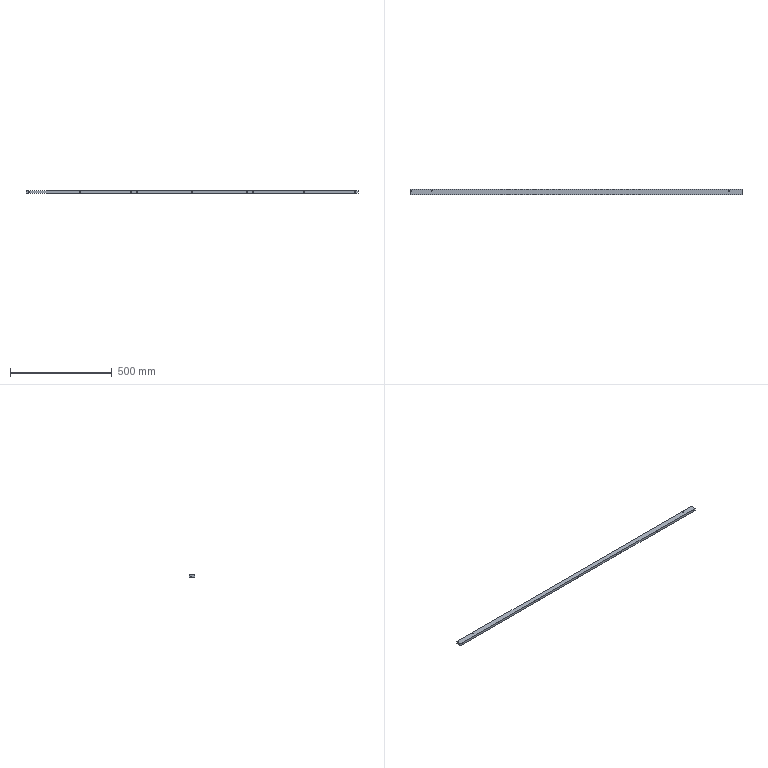Part | STEP file | J013-EBZ05-10-06 | 1 solid | 30 faces | box 1630 x 25 x 12 mm | volume 483875 mm3 | cylinder 24 | plane 6 | commonest cylinder face diameters 5 x24
STEP:
#1=CARTESIAN_POINT('',(1612.5,25.,6.));
#2=VERTEX_POINT('',#1);
#3=CARTESIAN_POINT('',(1617.5,25.,6.));
#4=VERTEX_POINT('',#3);
#5=CARTESIAN_POINT('',(1615.,25.,6.));
#6=DIRECTION('',(0.,-1.,0.));
#7=DIRECTION('',(1.,0.,0.));
#8=AXIS2_PLACEMENT_3D('',#5,#6,#7);
#9=CIRCLE('',#8,2.5);
#10=EDGE_CURVE('',#2,#4,#9,.T.);
#11=ORIENTED_EDGE('',*,*,#10,.F.);
#12=CARTESIAN_POINT('',(1612.5,0.,6.));
#13=VERTEX_POINT('',#12);
#14=CARTESIAN_POINT('',(1612.5,25.,6.));
#15=DIRECTION('',(0.,-1.,0.));
#16=VECTOR('',#15,1000.);
#17=LINE('',#14,#16);
#18=EDGE_CURVE('',#2,#13,#17,.T.);
#19=ORIENTED_EDGE('',*,*,#18,.T.);
#20=CARTESIAN_POINT('',(1617.5,0.,6.));
#21=VERTEX_POINT('',#20);
#22=CARTESIAN_POINT('',(1615.,0.,6.));
#23=DIRECTION('',(0.,1.,0.));
#24=DIRECTION('',(-1.,0.,0.));
#25=AXIS2_PLACEMENT_3D('',#22,#23,#24);
#26=CIRCLE('',#25,2.5);
#27=EDGE_CURVE('',#21,#13,#26,.T.);
#28=ORIENTED_EDGE('',*,*,#27,.F.);
#29=CARTESIAN_POINT('',(1617.5,25.,6.));
#30=DIRECTION('',(0.,-1.,0.));
#31=VECTOR('',#30,1000.);
#32=LINE('',#29,#31);
#33=EDGE_CURVE('',#4,#21,#32,.T.);
#34=ORIENTED_EDGE('',*,*,#33,.F.);
#35=EDGE_LOOP('',(#11,#19,#28,#34));
#36=FACE_OUTER_BOUND('',#35,.T.);
#37=CARTESIAN_POINT('',(1615.,25.,6.));
#38=DIRECTION('',(0.,-1.,0.));
#39=DIRECTION('',(1.,0.,0.));
#40=AXIS2_PLACEMENT_3D('',#37,#38,#39);
#41=CYLINDRICAL_SURFACE('',#40,2.5);
#42=ADVANCED_FACE('',(#36),#41,.F.);
#43=CARTESIAN_POINT('',(1362.5,25.,6.));
#44=VERTEX_POINT('',#43);
#45=CARTESIAN_POINT('',(1367.5,25.,6.));
#46=VERTEX_POINT('',#45);
#47=CARTESIAN_POINT('',(1365.,25.,6.));
#48=DIRECTION('',(0.,-1.,0.));
#49=DIRECTION('',(1.,0.,0.));
#50=AXIS2_PLACEMENT_3D('',#47,#48,#49);
#51=CIRCLE('',#50,2.5);
#52=EDGE_CURVE('',#44,#46,#51,.T.);
#53=ORIENTED_EDGE('',*,*,#52,.F.);
#54=CARTESIAN_POINT('',(1362.5,0.,6.));
#55=VERTEX_POINT('',#54);
#56=CARTESIAN_POINT('',(1362.5,25.,6.));
#57=DIRECTION('',(0.,-1.,0.));
#58=VECTOR('',#57,1000.);
#59=LINE('',#56,#58);
#60=EDGE_CURVE('',#44,#55,#59,.T.);
#61=ORIENTED_EDGE('',*,*,#60,.T.);
#62=CARTESIAN_POINT('',(1367.5,0.,6.));
#63=VERTEX_POINT('',#62);
#64=CARTESIAN_POINT('',(1365.,0.,6.));
#65=DIRECTION('',(0.,1.,0.));
#66=DIRECTION('',(-1.,0.,0.));
#67=AXIS2_PLACEMENT_3D('',#64,#65,#66);
#68=CIRCLE('',#67,2.5);
#69=EDGE_CURVE('',#63,#55,#68,.T.);
#70=ORIENTED_EDGE('',*,*,#69,.F.);
#71=CARTESIAN_POINT('',(1367.5,25.,6.));
#72=DIRECTION('',(0.,-1.,0.));
#73=VECTOR('',#72,1000.);
#74=LINE('',#71,#73);
#75=EDGE_CURVE('',#46,#63,#74,.T.);
#76=ORIENTED_EDGE('',*,*,#75,.F.);
#77=EDGE_LOOP('',(#53,#61,#70,#76));
#78=FACE_OUTER_BOUND('',#77,.T.);
#79=CARTESIAN_POINT('',(1365.,25.,6.));
#80=DIRECTION('',(0.,-1.,0.));
#81=DIRECTION('',(1.,0.,0.));
#82=AXIS2_PLACEMENT_3D('',#79,#80,#81);
#83=CYLINDRICAL_SURFACE('',#82,2.5);
#84=ADVANCED_FACE('',(#78),#83,.F.);
#85=CARTESIAN_POINT('',(1112.5,25.,6.));
#86=VERTEX_POINT('',#85);
#87=CARTESIAN_POINT('',(1117.5,25.,6.));
#88=VERTEX_POINT('',#87);
#89=CARTESIAN_POINT('',(1115.,25.,6.));
#90=DIRECTION('',(0.,-1.,0.));
#91=DIRECTION('',(1.,0.,0.));
#92=AXIS2_PLACEMENT_3D('',#89,#90,#91);
#93=CIRCLE('',#92,2.5);
#94=EDGE_CURVE('',#86,#88,#93,.T.);
#95=ORIENTED_EDGE('',*,*,#94,.F.);
#96=CARTESIAN_POINT('',(1112.5,0.,6.));
#97=VERTEX_POINT('',#96);
#98=CARTESIAN_POINT('',(1112.5,25.,6.));
#99=DIRECTION('',(0.,-1.,0.));
#100=VECTOR('',#99,1000.);
#101=LINE('',#98,#100);
#102=EDGE_CURVE('',#86,#97,#101,.T.);
#103=ORIENTED_EDGE('',*,*,#102,.T.);
#104=CARTESIAN_POINT('',(1117.5,0.,6.));
#105=VERTEX_POINT('',#104);
#106=CARTESIAN_POINT('',(1115.,0.,6.));
#107=DIRECTION('',(0.,1.,0.));
#108=DIRECTION('',(-1.,0.,0.));
#109=AXIS2_PLACEMENT_3D('',#106,#107,#108);
#110=CIRCLE('',#109,2.5);
#111=EDGE_CURVE('',#105,#97,#110,.T.);
#112=ORIENTED_EDGE('',*,*,#111,.F.);
#113=CARTESIAN_POINT('',(1117.5,25.,6.));
#114=DIRECTION('',(0.,-1.,0.));
#115=VECTOR('',#114,1000.);
#116=LINE('',#113,#115);
#117=EDGE_CURVE('',#88,#105,#116,.T.);
#118=ORIENTED_EDGE('',*,*,#117,.F.);
#119=EDGE_LOOP('',(#95,#103,#112,#118));
#120=FACE_OUTER_BOUND('',#119,.T.);
#121=CARTESIAN_POINT('',(1115.,25.,6.));
#122=DIRECTION('',(0.,-1.,0.));
#123=DIRECTION('',(1.,0.,0.));
#124=AXIS2_PLACEMENT_3D('',#121,#122,#123);
#125=CYLINDRICAL_SURFACE('',#124,2.5);
#126=ADVANCED_FACE('',(#120),#125,.F.);
#127=CARTESIAN_POINT('',(1082.5,25.,6.));
#128=VERTEX_POINT('',#127);
#129=CARTESIAN_POINT('',(1087.5,25.,6.));
#130=VERTEX_POINT('',#129);
#131=CARTESIAN_POINT('',(1085.,25.,6.));
#132=DIRECTION('',(0.,-1.,0.));
#133=DIRECTION('',(1.,0.,0.));
#134=AXIS2_PLACEMENT_3D('',#131,#132,#133);
#135=CIRCLE('',#134,2.5);
#136=EDGE_CURVE('',#128,#130,#135,.T.);
#137=ORIENTED_EDGE('',*,*,#136,.F.);
#138=CARTESIAN_POINT('',(1082.5,0.,6.));
#139=VERTEX_POINT('',#138);
#140=CARTESIAN_POINT('',(1082.5,25.,6.));
#141=DIRECTION('',(0.,-1.,0.));
#142=VECTOR('',#141,1000.);
#143=LINE('',#140,#142);
#144=EDGE_CURVE('',#128,#139,#143,.T.);
#145=ORIENTED_EDGE('',*,*,#144,.T.);
#146=CARTESIAN_POINT('',(1087.5,0.,6.));
#147=VERTEX_POINT('',#146);
#148=CARTESIAN_POINT('',(1085.,0.,6.));
#149=DIRECTION('',(0.,1.,0.));
#150=DIRECTION('',(-1.,0.,0.));
#151=AXIS2_PLACEMENT_3D('',#148,#149,#150);
#152=CIRCLE('',#151,2.5);
#153=EDGE_CURVE('',#147,#139,#152,.T.);
#154=ORIENTED_EDGE('',*,*,#153,.F.);
#155=CARTESIAN_POINT('',(1087.5,25.,6.));
#156=DIRECTION('',(0.,-1.,0.));
#157=VECTOR('',#156,1000.);
#158=LINE('',#155,#157);
#159=EDGE_CURVE('',#130,#147,#158,.T.);
#160=ORIENTED_EDGE('',*,*,#159,.F.);
#161=EDGE_LOOP('',(#137,#145,#154,#160));
#162=FACE_OUTER_BOUND('',#161,.T.);
#163=CARTESIAN_POINT('',(1085.,25.,6.));
#164=DIRECTION('',(0.,-1.,0.));
#165=DIRECTION('',(1.,0.,0.));
#166=AXIS2_PLACEMENT_3D('',#163,#164,#165);
#167=CYLINDRICAL_SURFACE('',#166,2.5);
#168=ADVANCED_FACE('',(#162),#167,.F.);
#169=CARTESIAN_POINT('',(812.5,25.,6.));
#170=VERTEX_POINT('',#169);
#171=CARTESIAN_POINT('',(817.5,25.,6.));
#172=VERTEX_POINT('',#171);
#173=CARTESIAN_POINT('',(815.,25.,6.));
#174=DIRECTION('',(0.,-1.,0.));
#175=DIRECTION('',(1.,0.,0.));
#176=AXIS2_PLACEMENT_3D('',#173,#174,#175);
#177=CIRCLE('',#176,2.5);
#178=EDGE_CURVE('',#170,#172,#177,.T.);
#179=ORIENTED_EDGE('',*,*,#178,.F.);
#180=CARTESIAN_POINT('',(812.5,0.,6.));
#181=VERTEX_POINT('',#180);
#182=CARTESIAN_POINT('',(812.5,25.,6.));
#183=DIRECTION('',(0.,-1.,0.));
#184=VECTOR('',#183,1000.);
#185=LINE('',#182,#184);
#186=EDGE_CURVE('',#170,#181,#185,.T.);
#187=ORIENTED_EDGE('',*,*,#186,.T.);
#188=CARTESIAN_POINT('',(817.5,0.,6.));
#189=VERTEX_POINT('',#188);
#190=CARTESIAN_POINT('',(815.,0.,6.));
#191=DIRECTION('',(0.,1.,0.));
#192=DIRECTION('',(-1.,0.,0.));
#193=AXIS2_PLACEMENT_3D('',#190,#191,#192);
#194=CIRCLE('',#193,2.5);
#195=EDGE_CURVE('',#189,#181,#194,.T.);
#196=ORIENTED_EDGE('',*,*,#195,.F.);
#197=CARTESIAN_POINT('',(817.5,25.,6.));
#198=DIRECTION('',(0.,-1.,0.));
#199=VECTOR('',#198,1000.);
#200=LINE('',#197,#199);
#201=EDGE_CURVE('',#172,#189,#200,.T.);
#202=ORIENTED_EDGE('',*,*,#201,.F.);
#203=EDGE_LOOP('',(#179,#187,#196,#202));
#204=FACE_OUTER_BOUND('',#203,.T.);
#205=CARTESIAN_POINT('',(815.,25.,6.));
#206=DIRECTION('',(0.,-1.,0.));
#207=DIRECTION('',(1.,0.,0.));
#208=AXIS2_PLACEMENT_3D('',#205,#206,#207);
#209=CYLINDRICAL_SURFACE('',#208,2.5);
#210=ADVANCED_FACE('',(#204),#209,.F.);
#211=CARTESIAN_POINT('',(542.5,25.,6.));
#212=VERTEX_POINT('',#211);
#213=CARTESIAN_POINT('',(547.5,25.,6.));
#214=VERTEX_POINT('',#213);
#215=CARTESIAN_POINT('',(545.,25.,6.));
#216=DIRECTION('',(0.,-1.,0.));
#217=DIRECTION('',(1.,0.,0.));
#218=AXIS2_PLACEMENT_3D('',#215,#216,#217);
#219=CIRCLE('',#218,2.5);
#220=EDGE_CURVE('',#212,#214,#219,.T.);
#221=ORIENTED_EDGE('',*,*,#220,.F.);
#222=CARTESIAN_POINT('',(542.5,0.,6.));
#223=VERTEX_POINT('',#222);
#224=CARTESIAN_POINT('',(542.5,25.,6.));
#225=DIRECTION('',(0.,-1.,0.));
#226=VECTOR('',#225,1000.);
#227=LINE('',#224,#226);
#228=EDGE_CURVE('',#212,#223,#227,.T.);
#229=ORIENTED_EDGE('',*,*,#228,.T.);
#230=CARTESIAN_POINT('',(547.5,0.,6.));
#231=VERTEX_POINT('',#230);
#232=CARTESIAN_POINT('',(545.,0.,6.));
#233=DIRECTION('',(0.,1.,0.));
#234=DIRECTION('',(-1.,0.,0.));
#235=AXIS2_PLACEMENT_3D('',#232,#233,#234);
#236=CIRCLE('',#235,2.5);
#237=EDGE_CURVE('',#231,#223,#236,.T.);
#238=ORIENTED_EDGE('',*,*,#237,.F.);
#239=CARTESIAN_POINT('',(547.5,25.,6.));
#240=DIRECTION('',(0.,-1.,0.));
#241=VECTOR('',#240,1000.);
#242=LINE('',#239,#241);
#243=EDGE_CURVE('',#214,#231,#242,.T.);
#244=ORIENTED_EDGE('',*,*,#243,.F.);
#245=EDGE_LOOP('',(#221,#229,#238,#244));
#246=FACE_OUTER_BOUND('',#245,.T.);
#247=CARTESIAN_POINT('',(545.,25.,6.));
#248=DIRECTION('',(0.,-1.,0.));
#249=DIRECTION('',(1.,0.,0.));
#250=AXIS2_PLACEMENT_3D('',#247,#248,#249);
#251=CYLINDRICAL_SURFACE('',#250,2.5);
#252=ADVANCED_FACE('',(#246),#251,.F.);
#253=CARTESIAN_POINT('',(512.5,25.,6.));
#254=VERTEX_POINT('',#253);
#255=CARTESIAN_POINT('',(517.5,25.,6.));
#256=VERTEX_POINT('',#255);
#257=CARTESIAN_POINT('',(515.,25.,6.));
#258=DIRECTION('',(0.,-1.,0.));
#259=DIRECTION('',(1.,0.,0.));
#260=AXIS2_PLACEMENT_3D('',#257,#258,#259);
#261=CIRCLE('',#260,2.5);
#262=EDGE_CURVE('',#254,#256,#261,.T.);
#263=ORIENTED_EDGE('',*,*,#262,.F.);
#264=CARTESIAN_POINT('',(512.5,0.,6.));
#265=VERTEX_POINT('',#264);
#266=CARTESIAN_POINT('',(512.5,25.,6.));
#267=DIRECTION('',(0.,-1.,0.));
#268=VECTOR('',#267,1000.);
#269=LINE('',#266,#268);
#270=EDGE_CURVE('',#254,#265,#269,.T.);
#271=ORIENTED_EDGE('',*,*,#270,.T.);
#272=CARTESIAN_POINT('',(517.5,0.,6.));
#273=VERTEX_POINT('',#272);
#274=CARTESIAN_POINT('',(515.,0.,6.));
#275=DIRECTION('',(0.,1.,0.));
#276=DIRECTION('',(-1.,0.,0.));
#277=AXIS2_PLACEMENT_3D('',#274,#275,#276);
#278=CIRCLE('',#277,2.5);
#279=EDGE_CURVE('',#273,#265,#278,.T.);
#280=ORIENTED_EDGE('',*,*,#279,.F.);
#281=CARTESIAN_POINT('',(517.5,25.,6.));
#282=DIRECTION('',(0.,-1.,0.));
#283=VECTOR('',#282,1000.);
#284=LINE('',#281,#283);
#285=EDGE_CURVE('',#256,#273,#284,.T.);
#286=ORIENTED_EDGE('',*,*,#285,.F.);
#287=EDGE_LOOP('',(#263,#271,#280,#286));
#288=FACE_OUTER_BOUND('',#287,.T.);
#289=CARTESIAN_POINT('',(515.,25.,6.));
#290=DIRECTION('',(0.,-1.,0.));
#291=DIRECTION('',(1.,0.,0.));
#292=AXIS2_PLACEMENT_3D('',#289,#290,#291);
#293=CYLINDRICAL_SURFACE('',#292,2.5);
#294=ADVANCED_FACE('',(#288),#293,.F.);
#295=CARTESIAN_POINT('',(262.5,25.,6.));
#296=VERTEX_POINT('',#295);
#297=CARTESIAN_POINT('',(267.5,25.,6.));
#298=VERTEX_POINT('',#297);
#299=CARTESIAN_POINT('',(265.,25.,6.));
#300=DIRECTION('',(0.,-1.,0.));
#301=DIRECTION('',(1.,0.,0.));
#302=AXIS2_PLACEMENT_3D('',#299,#300,#301);
#303=CIRCLE('',#302,2.5);
#304=EDGE_CURVE('',#296,#298,#303,.T.);
#305=ORIENTED_EDGE('',*,*,#304,.F.);
#306=CARTESIAN_POINT('',(262.5,0.,6.));
#307=VERTEX_POINT('',#306);
#308=CARTESIAN_POINT('',(262.5,25.,6.));
#309=DIRECTION('',(0.,-1.,0.));
#310=VECTOR('',#309,1000.);
#311=LINE('',#308,#310);
#312=EDGE_CURVE('',#296,#307,#311,.T.);
#313=ORIENTED_EDGE('',*,*,#312,.T.);
#314=CARTESIAN_POINT('',(267.5,0.,6.));
#315=VERTEX_POINT('',#314);
#316=CARTESIAN_POINT('',(265.,0.,6.));
#317=DIRECTION('',(0.,1.,0.));
#318=DIRECTION('',(-1.,0.,0.));
#319=AXIS2_PLACEMENT_3D('',#316,#317,#318);
#320=CIRCLE('',#319,2.5);
#321=EDGE_CURVE('',#315,#307,#320,.T.);
#322=ORIENTED_EDGE('',*,*,#321,.F.);
#323=CARTESIAN_POINT('',(267.5,25.,6.));
#324=DIRECTION('',(0.,-1.,0.));
#325=VECTOR('',#324,1000.);
#326=LINE('',#323,#325);
#327=EDGE_CURVE('',#298,#315,#326,.T.);
#328=ORIENTED_EDGE('',*,*,#327,.F.);
#329=EDGE_LOOP('',(#305,#313,#322,#328));
#330=FACE_OUTER_BOUND('',#329,.T.);
#331=CARTESIAN_POINT('',(265.,25.,6.));
#332=DIRECTION('',(0.,-1.,0.));
#333=DIRECTION('',(1.,0.,0.));
#334=AXIS2_PLACEMENT_3D('',#331,#332,#333);
#335=CYLINDRICAL_SURFACE('',#334,2.5);
#336=ADVANCED_FACE('',(#330),#335,.F.);
#337=CARTESIAN_POINT('',(1566.5,22.,0.));
#338=VERTEX_POINT('',#337);
#339=CARTESIAN_POINT('',(1566.5,17.,0.));
#340=VERTEX_POINT('',#339);
#341=CARTESIAN_POINT('',(1566.5,19.5,0.));
#342=DIRECTION('',(0.,0.,1.));
#343=DIRECTION('',(0.,-1.,0.));
#344=AXIS2_PLACEMENT_3D('',#341,#342,#343);
#345=CIRCLE('',#344,2.5);
#346=EDGE_CURVE('',#338,#340,#345,.T.);
#347=ORIENTED_EDGE('',*,*,#346,.F.);
#348=CARTESIAN_POINT('',(1566.5,22.,12.));
#349=VERTEX_POINT('',#348);
#350=CARTESIAN_POINT('',(1566.5,22.,0.));
#351=DIRECTION('',(0.,0.,1.));
#352=VECTOR('',#351,1000.);
#353=LINE('',#350,#352);
#354=EDGE_CURVE('',#338,#349,#353,.T.);
#355=ORIENTED_EDGE('',*,*,#354,.T.);
#356=CARTESIAN_POINT('',(1566.5,17.,12.));
#357=VERTEX_POINT('',#356);
#358=CARTESIAN_POINT('',(1566.5,19.5,12.));
#359=DIRECTION('',(0.,0.,-1.));
#360=DIRECTION('',(0.,1.,0.));
#361=AXIS2_PLACEMENT_3D('',#358,#359,#360);
#362=CIRCLE('',#361,2.5);
#363=EDGE_CURVE('',#357,#349,#362,.T.);
#364=ORIENTED_EDGE('',*,*,#363,.F.);
#365=CARTESIAN_POINT('',(1566.5,17.,0.));
#366=DIRECTION('',(0.,0.,1.));
#367=VECTOR('',#366,1000.);
#368=LINE('',#365,#367);
#369=EDGE_CURVE('',#340,#357,#368,.T.);
#370=ORIENTED_EDGE('',*,*,#369,.F.);
#371=EDGE_LOOP('',(#347,#355,#364,#370));
#372=FACE_OUTER_BOUND('',#371,.T.);
#373=CARTESIAN_POINT('',(1566.5,19.5,0.));
#374=DIRECTION('',(0.,0.,1.));
#375=DIRECTION('',(0.,-1.,0.));
#376=AXIS2_PLACEMENT_3D('',#373,#374,#375);
#377=CYLINDRICAL_SURFACE('',#376,2.5);
#378=ADVANCED_FACE('',(#372),#377,.F.);
#379=CARTESIAN_POINT('',(6.,22.,0.));
#380=VERTEX_POINT('',#379);
#381=CARTESIAN_POINT('',(6.,17.,0.));
#382=VERTEX_POINT('',#381);
#383=CARTESIAN_POINT('',(6.,19.5,0.));
#384=DIRECTION('',(0.,0.,1.));
#385=DIRECTION('',(0.,-1.,0.));
#386=AXIS2_PLACEMENT_3D('',#383,#384,#385);
#387=CIRCLE('',#386,2.5);
#388=EDGE_CURVE('',#380,#382,#387,.T.);
#389=ORIENTED_EDGE('',*,*,#388,.F.);
#390=CARTESIAN_POINT('',(6.,22.,12.));
#391=VERTEX_POINT('',#390);
#392=CARTESIAN_POINT('',(6.,22.,0.));
#393=DIRECTION('',(0.,0.,1.));
#394=VECTOR('',#393,1000.);
#395=LINE('',#392,#394);
#396=EDGE_CURVE('',#380,#391,#395,.T.);
#397=ORIENTED_EDGE('',*,*,#396,.T.);
#398=CARTESIAN_POINT('',(6.,17.,12.));
#399=VERTEX_POINT('',#398);
#400=CARTESIAN_POINT('',(6.,19.5,12.));
#401=DIRECTION('',(0.,0.,-1.));
#402=DIRECTION('',(0.,1.,0.));
#403=AXIS2_PLACEMENT_3D('',#400,#401,#402);
#404=CIRCLE('',#403,2.5);
#405=EDGE_CURVE('',#399,#391,#404,.T.);
#406=ORIENTED_EDGE('',*,*,#405,.F.);
#407=CARTESIAN_POINT('',(6.,17.,0.));
#408=DIRECTION('',(0.,0.,1.));
#409=VECTOR('',#408,1000.);
#410=LINE('',#407,#409);
#411=EDGE_CURVE('',#382,#399,#410,.T.);
#412=ORIENTED_EDGE('',*,*,#411,.F.);
#413=EDGE_LOOP('',(#389,#397,#406,#412));
#414=FACE_OUTER_BOUND('',#413,.T.);
#415=CARTESIAN_POINT('',(6.,19.5,0.));
#416=DIRECTION('',(0.,0.,1.));
#417=DIRECTION('',(0.,-1.,0.));
#418=AXIS2_PLACEMENT_3D('',#415,#416,#417);
#419=CYLINDRICAL_SURFACE('',#418,2.5);
#420=ADVANCED_FACE('',(#414),#419,.F.);
#421=CARTESIAN_POINT('',(106.,22.,0.));
#422=VERTEX_POINT('',#421);
#423=CARTESIAN_POINT('',(106.,17.,0.));
#424=VERTEX_POINT('',#423);
#425=CARTESIAN_POINT('',(106.,19.5,0.));
#426=DIRECTION('',(0.,0.,1.));
#427=DIRECTION('',(0.,-1.,0.));
#428=AXIS2_PLACEMENT_3D('',#425,#426,#427);
#429=CIRCLE('',#428,2.5);
#430=EDGE_CURVE('',#422,#424,#429,.T.);
#431=ORIENTED_EDGE('',*,*,#430,.F.);
#432=CARTESIAN_POINT('',(106.,22.,12.));
#433=VERTEX_POINT('',#432);
#434=CARTESIAN_POINT('',(106.,22.,0.));
#435=DIRECTION('',(0.,0.,1.));
#436=VECTOR('',#435,1000.);
#437=LINE('',#434,#436);
#438=EDGE_CURVE('',#422,#433,#437,.T.);
#439=ORIENTED_EDGE('',*,*,#438,.T.);
#440=CARTESIAN_POINT('',(106.,17.,12.));
#441=VERTEX_POINT('',#440);
#442=CARTESIAN_POINT('',(106.,19.5,12.));
#443=DIRECTION('',(0.,0.,-1.));
#444=DIRECTION('',(0.,1.,0.));
#445=AXIS2_PLACEMENT_3D('',#442,#443,#444);
#446=CIRCLE('',#445,2.5);
#447=EDGE_CURVE('',#441,#433,#446,.T.);
#448=ORIENTED_EDGE('',*,*,#447,.F.);
#449=CARTESIAN_POINT('',(106.,17.,0.));
#450=DIRECTION('',(0.,0.,1.));
#451=VECTOR('',#450,1000.);
#452=LINE('',#449,#451);
#453=EDGE_CURVE('',#424,#441,#452,.T.);
#454=ORIENTED_EDGE('',*,*,#453,.F.);
#455=EDGE_LOOP('',(#431,#439,#448,#454));
#456=FACE_OUTER_BOUND('',#455,.T.);
#457=CARTESIAN_POINT('',(106.,19.5,0.));
#458=DIRECTION('',(0.,0.,1.));
#459=DIRECTION('',(0.,-1.,0.));
#460=AXIS2_PLACEMENT_3D('',#457,#458,#459);
#461=CYLINDRICAL_SURFACE('',#460,2.5);
#462=ADVANCED_FACE('',(#456),#461,.F.);
#463=CARTESIAN_POINT('',(12.5,25.,6.));
#464=VERTEX_POINT('',#463);
#465=CARTESIAN_POINT('',(17.5,25.,6.));
#466=VERTEX_POINT('',#465);
#467=CARTESIAN_POINT('',(15.,25.,6.));
#468=DIRECTION('',(0.,-1.,0.));
#469=DIRECTION('',(1.,0.,0.));
#470=AXIS2_PLACEMENT_3D('',#467,#468,#469);
#471=CIRCLE('',#470,2.5);
#472=EDGE_CURVE('',#464,#466,#471,.T.);
#473=ORIENTED_EDGE('',*,*,#472,.F.);
#474=CARTESIAN_POINT('',(12.5,0.,6.));
#475=VERTEX_POINT('',#474);
#476=CARTESIAN_POINT('',(12.5,25.,6.));
#477=DIRECTION('',(0.,-1.,0.));
#478=VECTOR('',#477,1000.);
#479=LINE('',#476,#478);
#480=EDGE_CURVE('',#464,#475,#479,.T.);
#481=ORIENTED_EDGE('',*,*,#480,.T.);
#482=CARTESIAN_POINT('',(17.5,0.,6.));
#483=VERTEX_POINT('',#482);
#484=CARTESIAN_POINT('',(15.,0.,6.));
#485=DIRECTION('',(0.,1.,0.));
#486=DIRECTION('',(-1.,0.,0.));
#487=AXIS2_PLACEMENT_3D('',#484,#485,#486);
#488=CIRCLE('',#487,2.5);
#489=EDGE_CURVE('',#483,#475,#488,.T.);
#490=ORIENTED_EDGE('',*,*,#489,.F.);
#491=CARTESIAN_POINT('',(17.5,25.,6.));
#492=DIRECTION('',(0.,-1.,0.));
#493=VECTOR('',#492,1000.);
#494=LINE('',#491,#493);
#495=EDGE_CURVE('',#466,#483,#494,.T.);
#496=ORIENTED_EDGE('',*,*,#495,.F.);
#497=EDGE_LOOP('',(#473,#481,#490,#496));
#498=FACE_OUTER_BOUND('',#497,.T.);
#499=CARTESIAN_POINT('',(15.,25.,6.));
#500=DIRECTION('',(0.,-1.,0.));
#501=DIRECTION('',(1.,0.,0.));
#502=AXIS2_PLACEMENT_3D('',#499,#500,#501);
#503=CYLINDRICAL_SURFACE('',#502,2.5);
#504=ADVANCED_FACE('',(#498),#503,.F.);
#505=CARTESIAN_POINT('',(1615.,25.,6.));
#506=DIRECTION('',(0.,-1.,0.));
#507=DIRECTION('',(1.,0.,0.));
#508=AXIS2_PLACEMENT_3D('',#505,#506,#507);
#509=CIRCLE('',#508,2.5);
#510=EDGE_CURVE('',#4,#2,#509,.T.);
#511=ORIENTED_EDGE('',*,*,#510,.T.);
#512=ORIENTED_EDGE('',*,*,#10,.T.);
#513=EDGE_LOOP('',(#511,#512));
#514=FACE_BOUND('',#513,.T.);
#515=CARTESIAN_POINT('',(1365.,25.,6.));
#516=DIRECTION('',(0.,-1.,0.));
#517=DIRECTION('',(1.,0.,0.));
#518=AXIS2_PLACEMENT_3D('',#515,#516,#517);
#519=CIRCLE('',#518,2.5);
#520=EDGE_CURVE('',#46,#44,#519,.T.);
#521=ORIENTED_EDGE('',*,*,#520,.T.);
#522=ORIENTED_EDGE('',*,*,#52,.T.);
#523=EDGE_LOOP('',(#521,#522));
#524=FACE_BOUND('',#523,.T.);
#525=CARTESIAN_POINT('',(1115.,25.,6.));
#526=DIRECTION('',(0.,-1.,0.));
#527=DIRECTION('',(1.,0.,0.));
#528=AXIS2_PLACEMENT_3D('',#525,#526,#527);
#529=CIRCLE('',#528,2.5);
#530=EDGE_CURVE('',#88,#86,#529,.T.);
#531=ORIENTED_EDGE('',*,*,#530,.T.);
#532=ORIENTED_EDGE('',*,*,#94,.T.);
#533=EDGE_LOOP('',(#531,#532));
#534=FACE_BOUND('',#533,.T.);
#535=CARTESIAN_POINT('',(1085.,25.,6.));
#536=DIRECTION('',(0.,-1.,0.));
#537=DIRECTION('',(1.,0.,0.));
#538=AXIS2_PLACEMENT_3D('',#535,#536,#537);
#539=CIRCLE('',#538,2.5);
#540=EDGE_CURVE('',#130,#128,#539,.T.);
#541=ORIENTED_EDGE('',*,*,#540,.T.);
#542=ORIENTED_EDGE('',*,*,#136,.T.);
#543=EDGE_LOOP('',(#541,#542));
#544=FACE_BOUND('',#543,.T.);
#545=CARTESIAN_POINT('',(815.,25.,6.));
#546=DIRECTION('',(0.,-1.,0.));
#547=DIRECTION('',(1.,0.,0.));
#548=AXIS2_PLACEMENT_3D('',#545,#546,#547);
#549=CIRCLE('',#548,2.5);
#550=EDGE_CURVE('',#172,#170,#549,.T.);
#551=ORIENTED_EDGE('',*,*,#550,.T.);
#552=ORIENTED_EDGE('',*,*,#178,.T.);
#553=EDGE_LOOP('',(#551,#552));
#554=FACE_BOUND('',#553,.T.);
#555=CARTESIAN_POINT('',(545.,25.,6.));
#556=DIRECTION('',(0.,-1.,0.));
#557=DIRECTION('',(1.,0.,0.));
#558=AXIS2_PLACEMENT_3D('',#555,#556,#557);
#559=CIRCLE('',#558,2.5);
#560=EDGE_CURVE('',#214,#212,#559,.T.);
#561=ORIENTED_EDGE('',*,*,#560,.T.);
#562=ORIENTED_EDGE('',*,*,#220,.T.);
#563=EDGE_LOOP('',(#561,#562));
#564=FACE_BOUND('',#563,.T.);
#565=CARTESIAN_POINT('',(515.,25.,6.));
#566=DIRECTION('',(0.,-1.,0.));
#567=DIRECTION('',(1.,0.,0.));
#568=AXIS2_PLACEMENT_3D('',#565,#566,#567);
#569=CIRCLE('',#568,2.5);
#570=EDGE_CURVE('',#256,#254,#569,.T.);
#571=ORIENTED_EDGE('',*,*,#570,.T.);
#572=ORIENTED_EDGE('',*,*,#262,.T.);
#573=EDGE_LOOP('',(#571,#572));
#574=FACE_BOUND('',#573,.T.);
#575=CARTESIAN_POINT('',(265.,25.,6.));
#576=DIRECTION('',(0.,-1.,0.));
#577=DIRECTION('',(1.,0.,0.));
#578=AXIS2_PLACEMENT_3D('',#575,#576,#577);
#579=CIRCLE('',#578,2.5);
#580=EDGE_CURVE('',#298,#296,#579,.T.);
#581=ORIENTED_EDGE('',*,*,#580,.T.);
#582=ORIENTED_EDGE('',*,*,#304,.T.);
#583=EDGE_LOOP('',(#581,#582));
#584=FACE_BOUND('',#583,.T.);
#585=CARTESIAN_POINT('',(15.,25.,6.));
#586=DIRECTION('',(0.,-1.,0.));
#587=DIRECTION('',(1.,0.,0.));
#588=AXIS2_PLACEMENT_3D('',#585,#586,#587);
#589=CIRCLE('',#588,2.5);
#590=EDGE_CURVE('',#466,#464,#589,.T.);
#591=ORIENTED_EDGE('',*,*,#590,.T.);
#592=ORIENTED_EDGE('',*,*,#472,.T.);
#593=EDGE_LOOP('',(#591,#592));
#594=FACE_BOUND('',#593,.T.);
#595=CARTESIAN_POINT('',(0.,25.,12.));
#596=VERTEX_POINT('',#595);
#597=CARTESIAN_POINT('',(0.,25.,0.));
#598=VERTEX_POINT('',#597);
#599=CARTESIAN_POINT('',(0.,25.,6.));
#600=DIRECTION('',(0.,0.,-1.));
#601=VECTOR('',#600,1000.);
#602=LINE('',#599,#601);
#603=EDGE_CURVE('',#596,#598,#602,.T.);
#604=ORIENTED_EDGE('',*,*,#603,.F.);
#605=CARTESIAN_POINT('',(1630.,25.,12.));
#606=VERTEX_POINT('',#605);
#607=CARTESIAN_POINT('',(815.,25.,12.));
#608=DIRECTION('',(-1.,0.,0.));
#609=VECTOR('',#608,1000.);
#610=LINE('',#607,#609);
#611=EDGE_CURVE('',#606,#596,#610,.T.);
#612=ORIENTED_EDGE('',*,*,#611,.F.);
#613=CARTESIAN_POINT('',(1630.,25.,0.));
#614=VERTEX_POINT('',#613);
#615=CARTESIAN_POINT('',(1630.,25.,6.));
#616=DIRECTION('',(0.,0.,1.));
#617=VECTOR('',#616,1000.);
#618=LINE('',#615,#617);
#619=EDGE_CURVE('',#614,#606,#618,.T.);
#620=ORIENTED_EDGE('',*,*,#619,.F.);
#621=CARTESIAN_POINT('',(815.,25.,0.));
#622=DIRECTION('',(1.,0.,0.));
#623=VECTOR('',#622,1000.);
#624=LINE('',#621,#623);
#625=EDGE_CURVE('',#598,#614,#624,.T.);
#626=ORIENTED_EDGE('',*,*,#625,.F.);
#627=EDGE_LOOP('',(#604,#612,#620,#626));
#628=FACE_OUTER_BOUND('',#627,.T.);
#629=CARTESIAN_POINT('',(815.,25.,6.));
#630=DIRECTION('',(0.,1.,0.));
#631=DIRECTION('',(0.,0.,1.));
#632=AXIS2_PLACEMENT_3D('',#629,#630,#631);
#633=PLANE('',#632);
#634=ADVANCED_FACE('',(#514,#524,#534,#544,#554,#564,#574,#584,#594,#628),#633,.T.);
#635=CARTESIAN_POINT('',(0.,0.,12.));
#636=VERTEX_POINT('',#635);
#637=CARTESIAN_POINT('',(0.,0.,12.));
#638=DIRECTION('',(0.,1.,0.));
#639=VECTOR('',#638,1000.);
#640=LINE('',#637,#639);
#641=EDGE_CURVE('',#636,#596,#640,.T.);
#642=ORIENTED_EDGE('',*,*,#641,.T.);
#643=ORIENTED_EDGE('',*,*,#603,.T.);
#644=CARTESIAN_POINT('',(0.,0.,0.));
#645=VERTEX_POINT('',#644);
#646=CARTESIAN_POINT('',(0.,0.,0.));
#647=DIRECTION('',(0.,1.,0.));
#648=VECTOR('',#647,1000.);
#649=LINE('',#646,#648);
#650=EDGE_CURVE('',#645,#598,#649,.T.);
#651=ORIENTED_EDGE('',*,*,#650,.F.);
#652=CARTESIAN_POINT('',(0.,0.,6.));
#653=DIRECTION('',(0.,0.,1.));
#654=VECTOR('',#653,1000.);
#655=LINE('',#652,#654);
#656=EDGE_CURVE('',#645,#636,#655,.T.);
#657=ORIENTED_EDGE('',*,*,#656,.T.);
#658=EDGE_LOOP('',(#642,#643,#651,#657));
#659=FACE_OUTER_BOUND('',#658,.T.);
#660=CARTESIAN_POINT('',(0.,0.,6.));
#661=DIRECTION('',(-1.,0.,0.));
#662=DIRECTION('',(0.,-1.,0.));
#663=AXIS2_PLACEMENT_3D('',#660,#661,#662);
#664=PLANE('',#663);
#665=ADVANCED_FACE('',(#659),#664,.T.);
#666=CARTESIAN_POINT('',(1566.5,19.5,0.));
#667=DIRECTION('',(0.,0.,1.));
#668=DIRECTION('',(0.,-1.,0.));
#669=AXIS2_PLACEMENT_3D('',#666,#667,#668);
#670=CIRCLE('',#669,2.5);
#671=EDGE_CURVE('',#340,#338,#670,.T.);
#672=ORIENTED_EDGE('',*,*,#671,.T.);
#673=ORIENTED_EDGE('',*,*,#346,.T.);
#674=EDGE_LOOP('',(#672,#673));
#675=FACE_BOUND('',#674,.T.);
#676=CARTESIAN_POINT('',(6.,19.5,0.));
#677=DIRECTION('',(0.,0.,1.));
#678=DIRECTION('',(0.,-1.,0.));
#679=AXIS2_PLACEMENT_3D('',#676,#677,#678);
#680=CIRCLE('',#679,2.5);
#681=EDGE_CURVE('',#382,#380,#680,.T.);
#682=ORIENTED_EDGE('',*,*,#681,.T.);
#683=ORIENTED_EDGE('',*,*,#388,.T.);
#684=EDGE_LOOP('',(#682,#683));
#685=FACE_BOUND('',#684,.T.);
#686=CARTESIAN_POINT('',(106.,19.5,0.));
#687=DIRECTION('',(0.,0.,1.));
#688=DIRECTION('',(0.,-1.,0.));
#689=AXIS2_PLACEMENT_3D('',#686,#687,#688);
#690=CIRCLE('',#689,2.5);
#691=EDGE_CURVE('',#424,#422,#690,.T.);
#692=ORIENTED_EDGE('',*,*,#691,.T.);
#693=ORIENTED_EDGE('',*,*,#430,.T.);
#694=EDGE_LOOP('',(#692,#693));
#695=FACE_BOUND('',#694,.T.);
#696=ORIENTED_EDGE('',*,*,#650,.T.);
#697=ORIENTED_EDGE('',*,*,#625,.T.);
#698=CARTESIAN_POINT('',(1630.,0.,0.));
#699=VERTEX_POINT('',#698);
#700=CARTESIAN_POINT('',(1630.,0.,0.));
#701=DIRECTION('',(0.,1.,0.));
#702=VECTOR('',#701,1000.);
#703=LINE('',#700,#702);
#704=EDGE_CURVE('',#699,#614,#703,.T.);
#705=ORIENTED_EDGE('',*,*,#704,.F.);
#706=CARTESIAN_POINT('',(815.,0.,0.));
#707=DIRECTION('',(-1.,0.,0.));
#708=VECTOR('',#707,1000.);
#709=LINE('',#706,#708);
#710=EDGE_CURVE('',#699,#645,#709,.T.);
#711=ORIENTED_EDGE('',*,*,#710,.T.);
#712=EDGE_LOOP('',(#696,#697,#705,#711));
#713=FACE_OUTER_BOUND('',#712,.T.);
#714=CARTESIAN_POINT('',(815.,0.,0.));
#715=DIRECTION('',(0.,0.,-1.));
#716=DIRECTION('',(0.,1.,0.));
#717=AXIS2_PLACEMENT_3D('',#714,#715,#716);
#718=PLANE('',#717);
#719=ADVANCED_FACE('',(#675,#685,#695,#713),#718,.T.);
#720=ORIENTED_EDGE('',*,*,#704,.T.);
#721=ORIENTED_EDGE('',*,*,#619,.T.);
#722=CARTESIAN_POINT('',(1630.,0.,12.));
#723=VERTEX_POINT('',#722);
#724=CARTESIAN_POINT('',(1630.,0.,12.));
#725=DIRECTION('',(0.,1.,0.));
#726=VECTOR('',#725,1000.);
#727=LINE('',#724,#726);
#728=EDGE_CURVE('',#723,#606,#727,.T.);
#729=ORIENTED_EDGE('',*,*,#728,.F.);
#730=CARTESIAN_POINT('',(1630.,0.,6.));
#731=DIRECTION('',(0.,0.,-1.));
#732=VECTOR('',#731,1000.);
#733=LINE('',#730,#732);
#734=EDGE_CURVE('',#723,#699,#733,.T.);
#735=ORIENTED_EDGE('',*,*,#734,.T.);
#736=EDGE_LOOP('',(#720,#721,#729,#735));
#737=FACE_OUTER_BOUND('',#736,.T.);
#738=CARTESIAN_POINT('',(1630.,0.,6.));
#739=DIRECTION('',(1.,0.,0.));
#740=DIRECTION('',(0.,1.,0.));
#741=AXIS2_PLACEMENT_3D('',#738,#739,#740);
#742=PLANE('',#741);
#743=ADVANCED_FACE('',(#737),#742,.T.);
#744=ORIENTED_EDGE('',*,*,#27,.T.);
#745=CARTESIAN_POINT('',(1615.,0.,6.));
#746=DIRECTION('',(0.,1.,0.));
#747=DIRECTION('',(-1.,0.,0.));
#748=AXIS2_PLACEMENT_3D('',#745,#746,#747);
#749=CIRCLE('',#748,2.5);
#750=EDGE_CURVE('',#13,#21,#749,.T.);
#751=ORIENTED_EDGE('',*,*,#750,.T.);
#752=EDGE_LOOP('',(#744,#751));
#753=FACE_BOUND('',#752,.T.);
#754=ORIENTED_EDGE('',*,*,#69,.T.);
#755=CARTESIAN_POINT('',(1365.,0.,6.));
#756=DIRECTION('',(0.,1.,0.));
#757=DIRECTION('',(-1.,0.,0.));
#758=AXIS2_PLACEMENT_3D('',#755,#756,#757);
#759=CIRCLE('',#758,2.5);
#760=EDGE_CURVE('',#55,#63,#759,.T.);
#761=ORIENTED_EDGE('',*,*,#760,.T.);
#762=EDGE_LOOP('',(#754,#761));
#763=FACE_BOUND('',#762,.T.);
#764=ORIENTED_EDGE('',*,*,#111,.T.);
#765=CARTESIAN_POINT('',(1115.,0.,6.));
#766=DIRECTION('',(0.,1.,0.));
#767=DIRECTION('',(-1.,0.,0.));
#768=AXIS2_PLACEMENT_3D('',#765,#766,#767);
#769=CIRCLE('',#768,2.5);
#770=EDGE_CURVE('',#97,#105,#769,.T.);
#771=ORIENTED_EDGE('',*,*,#770,.T.);
#772=EDGE_LOOP('',(#764,#771));
#773=FACE_BOUND('',#772,.T.);
#774=ORIENTED_EDGE('',*,*,#153,.T.);
#775=CARTESIAN_POINT('',(1085.,0.,6.));
#776=DIRECTION('',(0.,1.,0.));
#777=DIRECTION('',(-1.,0.,0.));
#778=AXIS2_PLACEMENT_3D('',#775,#776,#777);
#779=CIRCLE('',#778,2.5);
#780=EDGE_CURVE('',#139,#147,#779,.T.);
#781=ORIENTED_EDGE('',*,*,#780,.T.);
#782=EDGE_LOOP('',(#774,#781));
#783=FACE_BOUND('',#782,.T.);
#784=ORIENTED_EDGE('',*,*,#195,.T.);
#785=CARTESIAN_POINT('',(815.,0.,6.));
#786=DIRECTION('',(0.,1.,0.));
#787=DIRECTION('',(-1.,0.,0.));
#788=AXIS2_PLACEMENT_3D('',#785,#786,#787);
#789=CIRCLE('',#788,2.5);
#790=EDGE_CURVE('',#181,#189,#789,.T.);
#791=ORIENTED_EDGE('',*,*,#790,.T.);
#792=EDGE_LOOP('',(#784,#791));
#793=FACE_BOUND('',#792,.T.);
#794=ORIENTED_EDGE('',*,*,#237,.T.);
#795=CARTESIAN_POINT('',(545.,0.,6.));
#796=DIRECTION('',(0.,1.,0.));
#797=DIRECTION('',(-1.,0.,0.));
#798=AXIS2_PLACEMENT_3D('',#795,#796,#797);
#799=CIRCLE('',#798,2.5);
#800=EDGE_CURVE('',#223,#231,#799,.T.);
#801=ORIENTED_EDGE('',*,*,#800,.T.);
#802=EDGE_LOOP('',(#794,#801));
#803=FACE_BOUND('',#802,.T.);
#804=ORIENTED_EDGE('',*,*,#279,.T.);
#805=CARTESIAN_POINT('',(515.,0.,6.));
#806=DIRECTION('',(0.,1.,0.));
#807=DIRECTION('',(-1.,0.,0.));
#808=AXIS2_PLACEMENT_3D('',#805,#806,#807);
#809=CIRCLE('',#808,2.5);
#810=EDGE_CURVE('',#265,#273,#809,.T.);
#811=ORIENTED_EDGE('',*,*,#810,.T.);
#812=EDGE_LOOP('',(#804,#811));
#813=FACE_BOUND('',#812,.T.);
#814=ORIENTED_EDGE('',*,*,#321,.T.);
#815=CARTESIAN_POINT('',(265.,0.,6.));
#816=DIRECTION('',(0.,1.,0.));
#817=DIRECTION('',(-1.,0.,0.));
#818=AXIS2_PLACEMENT_3D('',#815,#816,#817);
#819=CIRCLE('',#818,2.5);
#820=EDGE_CURVE('',#307,#315,#819,.T.);
#821=ORIENTED_EDGE('',*,*,#820,.T.);
#822=EDGE_LOOP('',(#814,#821));
#823=FACE_BOUND('',#822,.T.);
#824=ORIENTED_EDGE('',*,*,#489,.T.);
#825=CARTESIAN_POINT('',(15.,0.,6.));
#826=DIRECTION('',(0.,1.,0.));
#827=DIRECTION('',(-1.,0.,0.));
#828=AXIS2_PLACEMENT_3D('',#825,#826,#827);
#829=CIRCLE('',#828,2.5);
#830=EDGE_CURVE('',#475,#483,#829,.T.);
#831=ORIENTED_EDGE('',*,*,#830,.T.);
#832=EDGE_LOOP('',(#824,#831));
#833=FACE_BOUND('',#832,.T.);
#834=CARTESIAN_POINT('',(815.,0.,12.));
#835=DIRECTION('',(1.,0.,0.));
#836=VECTOR('',#835,1000.);
#837=LINE('',#834,#836);
#838=EDGE_CURVE('',#636,#723,#837,.T.);
#839=ORIENTED_EDGE('',*,*,#838,.F.);
#840=ORIENTED_EDGE('',*,*,#656,.F.);
#841=ORIENTED_EDGE('',*,*,#710,.F.);
#842=ORIENTED_EDGE('',*,*,#734,.F.);
#843=EDGE_LOOP('',(#839,#840,#841,#842));
#844=FACE_OUTER_BOUND('',#843,.T.);
#845=CARTESIAN_POINT('',(815.,0.,6.));
#846=DIRECTION('',(0.,-1.,0.));
#847=DIRECTION('',(0.,0.,-1.));
#848=AXIS2_PLACEMENT_3D('',#845,#846,#847);
#849=PLANE('',#848);
#850=ADVANCED_FACE('',(#753,#763,#773,#783,#793,#803,#813,#823,#833,#844),#849,.T.);
#851=ORIENTED_EDGE('',*,*,#363,.T.);
#852=CARTESIAN_POINT('',(1566.5,19.5,12.));
#853=DIRECTION('',(0.,0.,-1.));
#854=DIRECTION('',(0.,1.,0.));
#855=AXIS2_PLACEMENT_3D('',#852,#853,#854);
#856=CIRCLE('',#855,2.5);
#857=EDGE_CURVE('',#349,#357,#856,.T.);
#858=ORIENTED_EDGE('',*,*,#857,.T.);
#859=EDGE_LOOP('',(#851,#858));
#860=FACE_BOUND('',#859,.T.);
#861=ORIENTED_EDGE('',*,*,#405,.T.);
#862=CARTESIAN_POINT('',(6.,19.5,12.));
#863=DIRECTION('',(0.,0.,-1.));
#864=DIRECTION('',(0.,1.,0.));
#865=AXIS2_PLACEMENT_3D('',#862,#863,#864);
#866=CIRCLE('',#865,2.5);
#867=EDGE_CURVE('',#391,#399,#866,.T.);
#868=ORIENTED_EDGE('',*,*,#867,.T.);
#869=EDGE_LOOP('',(#861,#868));
#870=FACE_BOUND('',#869,.T.);
#871=ORIENTED_EDGE('',*,*,#447,.T.);
#872=CARTESIAN_POINT('',(106.,19.5,12.));
#873=DIRECTION('',(0.,0.,-1.));
#874=DIRECTION('',(0.,1.,0.));
#875=AXIS2_PLACEMENT_3D('',#872,#873,#874);
#876=CIRCLE('',#875,2.5);
#877=EDGE_CURVE('',#433,#441,#876,.T.);
#878=ORIENTED_EDGE('',*,*,#877,.T.);
#879=EDGE_LOOP('',(#871,#878));
#880=FACE_BOUND('',#879,.T.);
#881=ORIENTED_EDGE('',*,*,#838,.T.);
#882=ORIENTED_EDGE('',*,*,#728,.T.);
#883=ORIENTED_EDGE('',*,*,#611,.T.);
#884=ORIENTED_EDGE('',*,*,#641,.F.);
#885=EDGE_LOOP('',(#881,#882,#883,#884));
#886=FACE_OUTER_BOUND('',#885,.T.);
#887=CARTESIAN_POINT('',(815.,0.,12.));
#888=DIRECTION('',(0.,0.,1.));
#889=DIRECTION('',(0.,-1.,0.));
#890=AXIS2_PLACEMENT_3D('',#887,#888,#889);
#891=PLANE('',#890);
#892=ADVANCED_FACE('',(#860,#870,#880,#886),#891,.T.);
#893=ORIENTED_EDGE('',*,*,#480,.F.);
#894=ORIENTED_EDGE('',*,*,#590,.F.);
#895=ORIENTED_EDGE('',*,*,#495,.T.);
#896=ORIENTED_EDGE('',*,*,#830,.F.);
#897=EDGE_LOOP('',(#893,#894,#895,#896));
#898=FACE_OUTER_BOUND('',#897,.T.);
#899=CARTESIAN_POINT('',(15.,25.,6.));
#900=DIRECTION('',(0.,-1.,0.));
#901=DIRECTION('',(1.,0.,0.));
#902=AXIS2_PLACEMENT_3D('',#899,#900,#901);
#903=CYLINDRICAL_SURFACE('',#902,2.5);
#904=ADVANCED_FACE('',(#898),#903,.F.);
#905=ORIENTED_EDGE('',*,*,#438,.F.);
#906=ORIENTED_EDGE('',*,*,#691,.F.);
#907=ORIENTED_EDGE('',*,*,#453,.T.);
#908=ORIENTED_EDGE('',*,*,#877,.F.);
#909=EDGE_LOOP('',(#905,#906,#907,#908));
#910=FACE_OUTER_BOUND('',#909,.T.);
#911=CARTESIAN_POINT('',(106.,19.5,0.));
#912=DIRECTION('',(0.,0.,1.));
#913=DIRECTION('',(0.,-1.,0.));
#914=AXIS2_PLACEMENT_3D('',#911,#912,#913);
#915=CYLINDRICAL_SURFACE('',#914,2.5);
#916=ADVANCED_FACE('',(#910),#915,.F.);
#917=ORIENTED_EDGE('',*,*,#396,.F.);
#918=ORIENTED_EDGE('',*,*,#681,.F.);
#919=ORIENTED_EDGE('',*,*,#411,.T.);
#920=ORIENTED_EDGE('',*,*,#867,.F.);
#921=EDGE_LOOP('',(#917,#918,#919,#920));
#922=FACE_OUTER_BOUND('',#921,.T.);
#923=CARTESIAN_POINT('',(6.,19.5,0.));
#924=DIRECTION('',(0.,0.,1.));
#925=DIRECTION('',(0.,-1.,0.));
#926=AXIS2_PLACEMENT_3D('',#923,#924,#925);
#927=CYLINDRICAL_SURFACE('',#926,2.5);
#928=ADVANCED_FACE('',(#922),#927,.F.);
#929=ORIENTED_EDGE('',*,*,#354,.F.);
#930=ORIENTED_EDGE('',*,*,#671,.F.);
#931=ORIENTED_EDGE('',*,*,#369,.T.);
#932=ORIENTED_EDGE('',*,*,#857,.F.);
#933=EDGE_LOOP('',(#929,#930,#931,#932));
#934=FACE_OUTER_BOUND('',#933,.T.);
#935=CARTESIAN_POINT('',(1566.5,19.5,0.));
#936=DIRECTION('',(0.,0.,1.));
#937=DIRECTION('',(0.,-1.,0.));
#938=AXIS2_PLACEMENT_3D('',#935,#936,#937);
#939=CYLINDRICAL_SURFACE('',#938,2.5);
#940=ADVANCED_FACE('',(#934),#939,.F.);
#941=ORIENTED_EDGE('',*,*,#312,.F.);
#942=ORIENTED_EDGE('',*,*,#580,.F.);
#943=ORIENTED_EDGE('',*,*,#327,.T.);
#944=ORIENTED_EDGE('',*,*,#820,.F.);
#945=EDGE_LOOP('',(#941,#942,#943,#944));
#946=FACE_OUTER_BOUND('',#945,.T.);
#947=CARTESIAN_POINT('',(265.,25.,6.));
#948=DIRECTION('',(0.,-1.,0.));
#949=DIRECTION('',(1.,0.,0.));
#950=AXIS2_PLACEMENT_3D('',#947,#948,#949);
#951=CYLINDRICAL_SURFACE('',#950,2.5);
#952=ADVANCED_FACE('',(#946),#951,.F.);
#953=ORIENTED_EDGE('',*,*,#270,.F.);
#954=ORIENTED_EDGE('',*,*,#570,.F.);
#955=ORIENTED_EDGE('',*,*,#285,.T.);
#956=ORIENTED_EDGE('',*,*,#810,.F.);
#957=EDGE_LOOP('',(#953,#954,#955,#956));
#958=FACE_OUTER_BOUND('',#957,.T.);
#959=CARTESIAN_POINT('',(515.,25.,6.));
#960=DIRECTION('',(0.,-1.,0.));
#961=DIRECTION('',(1.,0.,0.));
#962=AXIS2_PLACEMENT_3D('',#959,#960,#961);
#963=CYLINDRICAL_SURFACE('',#962,2.5);
#964=ADVANCED_FACE('',(#958),#963,.F.);
#965=ORIENTED_EDGE('',*,*,#228,.F.);
#966=ORIENTED_EDGE('',*,*,#560,.F.);
#967=ORIENTED_EDGE('',*,*,#243,.T.);
#968=ORIENTED_EDGE('',*,*,#800,.F.);
#969=EDGE_LOOP('',(#965,#966,#967,#968));
#970=FACE_OUTER_BOUND('',#969,.T.);
#971=CARTESIAN_POINT('',(545.,25.,6.));
#972=DIRECTION('',(0.,-1.,0.));
#973=DIRECTION('',(1.,0.,0.));
#974=AXIS2_PLACEMENT_3D('',#971,#972,#973);
#975=CYLINDRICAL_SURFACE('',#974,2.5);
#976=ADVANCED_FACE('',(#970),#975,.F.);
#977=ORIENTED_EDGE('',*,*,#186,.F.);
#978=ORIENTED_EDGE('',*,*,#550,.F.);
#979=ORIENTED_EDGE('',*,*,#201,.T.);
#980=ORIENTED_EDGE('',*,*,#790,.F.);
#981=EDGE_LOOP('',(#977,#978,#979,#980));
#982=FACE_OUTER_BOUND('',#981,.T.);
#983=CARTESIAN_POINT('',(815.,25.,6.));
#984=DIRECTION('',(0.,-1.,0.));
#985=DIRECTION('',(1.,0.,0.));
#986=AXIS2_PLACEMENT_3D('',#983,#984,#985);
#987=CYLINDRICAL_SURFACE('',#986,2.5);
#988=ADVANCED_FACE('',(#982),#987,.F.);
#989=ORIENTED_EDGE('',*,*,#144,.F.);
#990=ORIENTED_EDGE('',*,*,#540,.F.);
#991=ORIENTED_EDGE('',*,*,#159,.T.);
#992=ORIENTED_EDGE('',*,*,#780,.F.);
#993=EDGE_LOOP('',(#989,#990,#991,#992));
#994=FACE_OUTER_BOUND('',#993,.T.);
#995=CARTESIAN_POINT('',(1085.,25.,6.));
#996=DIRECTION('',(0.,-1.,0.));
#997=DIRECTION('',(1.,0.,0.));
#998=AXIS2_PLACEMENT_3D('',#995,#996,#997);
#999=CYLINDRICAL_SURFACE('',#998,2.5);
#1000=ADVANCED_FACE('',(#994),#999,.F.);
#1001=ORIENTED_EDGE('',*,*,#102,.F.);
#1002=ORIENTED_EDGE('',*,*,#530,.F.);
#1003=ORIENTED_EDGE('',*,*,#117,.T.);
#1004=ORIENTED_EDGE('',*,*,#770,.F.);
#1005=EDGE_LOOP('',(#1001,#1002,#1003,#1004));
#1006=FACE_OUTER_BOUND('',#1005,.T.);
#1007=CARTESIAN_POINT('',(1115.,25.,6.));
#1008=DIRECTION('',(0.,-1.,0.));
#1009=DIRECTION('',(1.,0.,0.));
#1010=AXIS2_PLACEMENT_3D('',#1007,#1008,#1009);
#1011=CYLINDRICAL_SURFACE('',#1010,2.5);
#1012=ADVANCED_FACE('',(#1006),#1011,.F.);
#1013=ORIENTED_EDGE('',*,*,#60,.F.);
#1014=ORIENTED_EDGE('',*,*,#520,.F.);
#1015=ORIENTED_EDGE('',*,*,#75,.T.);
#1016=ORIENTED_EDGE('',*,*,#760,.F.);
#1017=EDGE_LOOP('',(#1013,#1014,#1015,#1016));
#1018=FACE_OUTER_BOUND('',#1017,.T.);
#1019=CARTESIAN_POINT('',(1365.,25.,6.));
#1020=DIRECTION('',(0.,-1.,0.));
#1021=DIRECTION('',(1.,0.,0.));
#1022=AXIS2_PLACEMENT_3D('',#1019,#1020,#1021);
#1023=CYLINDRICAL_SURFACE('',#1022,2.5);
#1024=ADVANCED_FACE('',(#1018),#1023,.F.);
#1025=ORIENTED_EDGE('',*,*,#18,.F.);
#1026=ORIENTED_EDGE('',*,*,#510,.F.);
#1027=ORIENTED_EDGE('',*,*,#33,.T.);
#1028=ORIENTED_EDGE('',*,*,#750,.F.);
#1029=EDGE_LOOP('',(#1025,#1026,#1027,#1028));
#1030=FACE_OUTER_BOUND('',#1029,.T.);
#1031=CARTESIAN_POINT('',(1615.,25.,6.));
#1032=DIRECTION('',(0.,-1.,0.));
#1033=DIRECTION('',(1.,0.,0.));
#1034=AXIS2_PLACEMENT_3D('',#1031,#1032,#1033);
#1035=CYLINDRICAL_SURFACE('',#1034,2.5);
#1036=ADVANCED_FACE('',(#1030),#1035,.F.);
#1037=CLOSED_SHELL('',(#42,#84,#126,#168,#210,#252,#294,#336,#378,#420,#462,#504,#634,#665,#719,#743,#850,#892,#904,#916,#928,#940,#952,#964,#976,#988,#1000,#1012,#1024,#1036));
#1038=MANIFOLD_SOLID_BREP('',#1037);
#1039=CARTESIAN_POINT('',(0.,0.,0.));
#1040=DIRECTION('',(0.,0.,1.));
#1041=DIRECTION('',(1.,0.,0.));
#1042=AXIS2_PLACEMENT_3D('',#1039,#1040,#1041);
#1043=(LENGTH_UNIT()NAMED_UNIT(*)SI_UNIT(.MILLI.,.METRE.));
#1044=UNCERTAINTY_MEASURE_WITH_UNIT(LENGTH_MEASURE(0.00001),#1043,'','');
#1045=(NAMED_UNIT(*)PLANE_ANGLE_UNIT()SI_UNIT($,.RADIAN.));
#1046=(NAMED_UNIT(*)SI_UNIT($,.STERADIAN.)SOLID_ANGLE_UNIT());
#1047=(GEOMETRIC_REPRESENTATION_CONTEXT(3)GLOBAL_UNCERTAINTY_ASSIGNED_CONTEXT((#1044))GLOBAL_UNIT_ASSIGNED_CONTEXT((#1043,#1045,#1046))REPRESENTATION_CONTEXT('',''));
#1048=ADVANCED_BREP_SHAPE_REPRESENTATION('',(#1038,#1042),#1047);